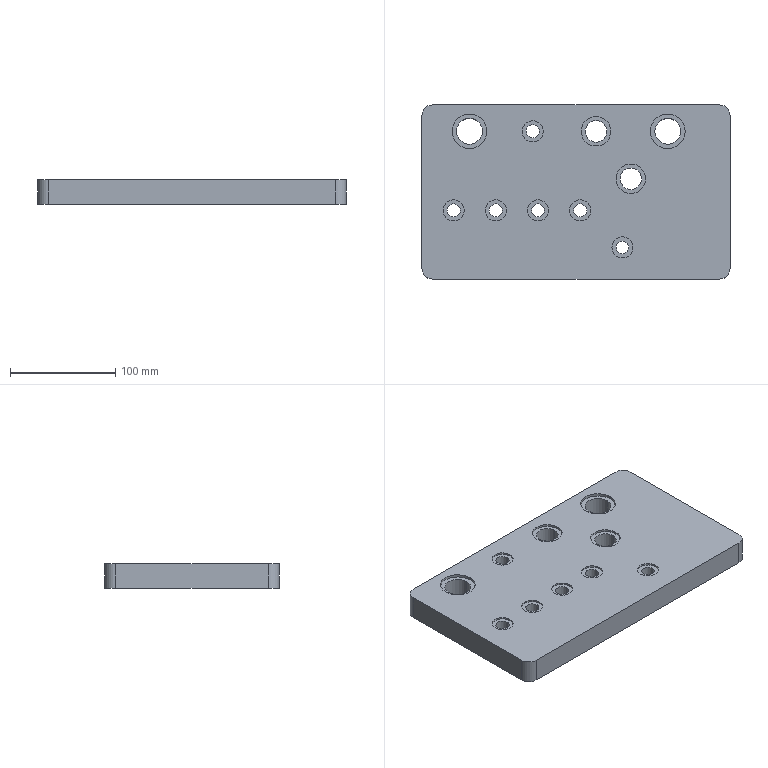Part | SolidWorks | features HoleWzd 4, ICE 3, FlatPattern 1, SMBaseFlange 1, SheetMetal 1 | 1 solid | 60 faces | box 292 x 165 x 23 mm | volume 1047864 mm3 | cylinder 44 | plane 16 | commonest cylinder face diameters 20 x16 12.5 x10 20.5 x4 24.5 x4 28 x4 33 x4